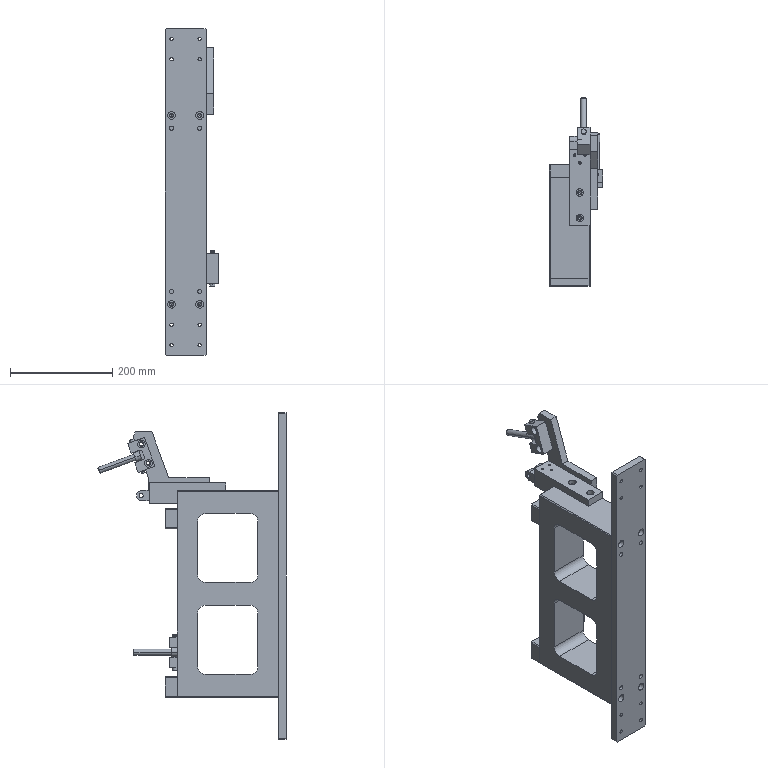Part | SolidWorks | 13 solids | 392 faces | box 105 x 368.457 x 640 mm | volume 5129898 mm3 | cylinder 214 | plane 138 | cone 40 | commonest cylinder face diameters 6.8 x38 15 x38 9 x30 6.6 x16 11 x16 8 x12